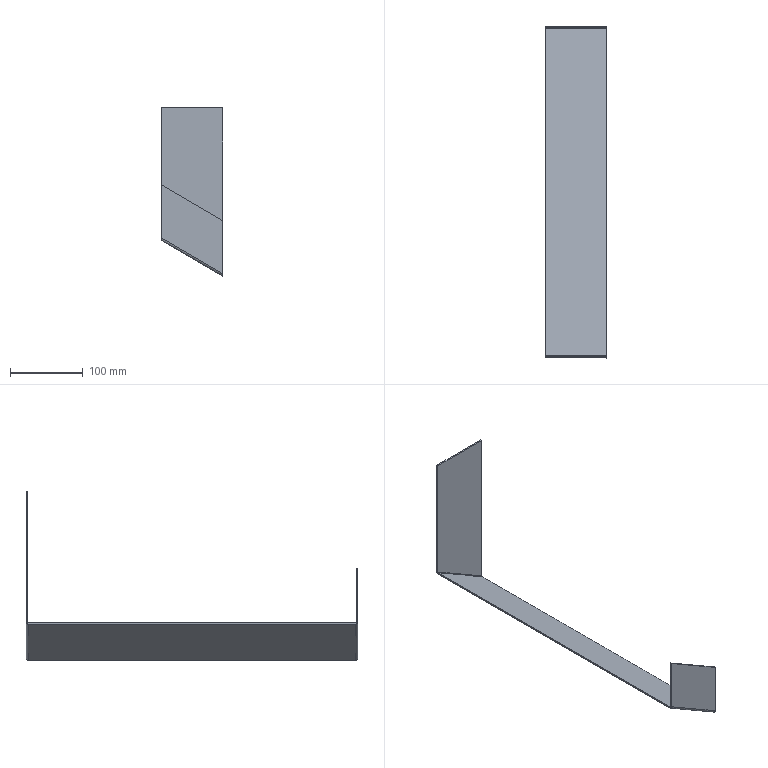Part | STEP file | lll_id4154_x_t | 1 solid | 14 faces | box 85 x 455 x 230.884 mm | volume 136229 mm3 | plane 10 | cylinder 4 | commonest cylinder face diameters 2 x2 6 x2
STEP:
#1=CARTESIAN_POINT('',(4052.435,-471.,-155.174));
#2=VERTEX_POINT('',#1);
#3=CARTESIAN_POINT('',(4052.435,-471.,-227.92));
#4=VERTEX_POINT('',#3);
#5=CARTESIAN_POINT('',(4052.435,-471.,-250.));
#6=DIRECTION('',(0.,0.,-1.));
#7=VECTOR('',#6,1.);
#8=LINE('',#5,#7);
#9=EDGE_CURVE('',#2,#4,#8,.T.);
#10=ORIENTED_EDGE('',*,*,#9,.T.);
#11=CARTESIAN_POINT('',(4052.435,-468.,-231.384));
#12=VERTEX_POINT('',#11);
#13=CARTESIAN_POINT('',(4052.435,-468.,-227.92));
#14=DIRECTION('',(1.,0.,0.));
#15=DIRECTION('',(0.,0.,-1.));
#16=AXIS2_PLACEMENT_3D('',#13,#14,#15);
#17=ELLIPSE('',#16,3.464,3.);
#18=EDGE_CURVE('',#4,#12,#17,.T.);
#19=ORIENTED_EDGE('',*,*,#18,.T.);
#20=CARTESIAN_POINT('',(4052.435,-19.,-231.384));
#21=VERTEX_POINT('',#20);
#22=CARTESIAN_POINT('',(4052.435,600.,-231.384));
#23=DIRECTION('',(0.,1.,0.));
#24=VECTOR('',#23,1.);
#25=LINE('',#22,#24);
#26=EDGE_CURVE('',#12,#21,#25,.T.);
#27=ORIENTED_EDGE('',*,*,#26,.T.);
#28=CARTESIAN_POINT('',(4052.435,-16.,-227.92));
#29=VERTEX_POINT('',#28);
#30=CARTESIAN_POINT('',(4052.435,-19.,-227.92));
#31=DIRECTION('',(1.,0.,0.));
#32=DIRECTION('',(0.,0.,-1.));
#33=AXIS2_PLACEMENT_3D('',#30,#31,#32);
#34=ELLIPSE('',#33,3.464,3.);
#35=EDGE_CURVE('',#21,#29,#34,.T.);
#36=ORIENTED_EDGE('',*,*,#35,.T.);
#37=CARTESIAN_POINT('',(4052.435,-16.,-0.5));
#38=VERTEX_POINT('',#37);
#39=CARTESIAN_POINT('',(4052.435,-16.,-131.405));
#40=DIRECTION('',(0.,0.,-1.));
#41=VECTOR('',#40,1.);
#42=LINE('',#39,#41);
#43=EDGE_CURVE('',#38,#29,#42,.T.);
#44=ORIENTED_EDGE('',*,*,#43,.F.);
#45=CARTESIAN_POINT('',(4052.435,-18.,-0.5));
#46=VERTEX_POINT('',#45);
#47=CARTESIAN_POINT('',(4052.435,-16.,-0.5));
#48=DIRECTION('',(0.,1.,0.));
#49=VECTOR('',#48,1.);
#50=LINE('',#47,#49);
#51=EDGE_CURVE('',#46,#38,#50,.T.);
#52=ORIENTED_EDGE('',*,*,#51,.F.);
#53=CARTESIAN_POINT('',(4052.435,-18.,-227.92));
#54=VERTEX_POINT('',#53);
#55=CARTESIAN_POINT('',(4052.435,-18.,-250.));
#56=DIRECTION('',(0.,0.,1.));
#57=VECTOR('',#56,1.);
#58=LINE('',#55,#57);
#59=EDGE_CURVE('',#54,#46,#58,.T.);
#60=ORIENTED_EDGE('',*,*,#59,.F.);
#61=CARTESIAN_POINT('',(4052.435,-19.,-229.075));
#62=VERTEX_POINT('',#61);
#63=CARTESIAN_POINT('',(4052.435,-19.,-227.92));
#64=DIRECTION('',(-1.,0.,0.));
#65=DIRECTION('',(0.,0.,1.));
#66=AXIS2_PLACEMENT_3D('',#63,#64,#65);
#67=ELLIPSE('',#66,1.155,1.);
#68=EDGE_CURVE('',#54,#62,#67,.T.);
#69=ORIENTED_EDGE('',*,*,#68,.T.);
#70=CARTESIAN_POINT('',(4052.435,-468.,-229.075));
#71=VERTEX_POINT('',#70);
#72=CARTESIAN_POINT('',(4052.435,600.,-229.075));
#73=DIRECTION('',(0.,1.,0.));
#74=VECTOR('',#73,1.);
#75=LINE('',#72,#74);
#76=EDGE_CURVE('',#71,#62,#75,.T.);
#77=ORIENTED_EDGE('',*,*,#76,.F.);
#78=CARTESIAN_POINT('',(4052.435,-469.,-227.92));
#79=VERTEX_POINT('',#78);
#80=CARTESIAN_POINT('',(4052.435,-468.,-227.92));
#81=DIRECTION('',(-1.,0.,0.));
#82=DIRECTION('',(0.,0.,1.));
#83=AXIS2_PLACEMENT_3D('',#80,#81,#82);
#84=ELLIPSE('',#83,1.155,1.);
#85=EDGE_CURVE('',#71,#79,#84,.T.);
#86=ORIENTED_EDGE('',*,*,#85,.T.);
#87=CARTESIAN_POINT('',(4052.435,-469.,-155.174));
#88=VERTEX_POINT('',#87);
#89=CARTESIAN_POINT('',(4052.435,-469.,-180.));
#90=DIRECTION('',(0.,0.,1.));
#91=VECTOR('',#90,1.);
#92=LINE('',#89,#91);
#93=EDGE_CURVE('',#79,#88,#92,.T.);
#94=ORIENTED_EDGE('',*,*,#93,.T.);
#95=CARTESIAN_POINT('',(4052.435,0.,-155.174));
#96=DIRECTION('',(0.,-1.,0.));
#97=VECTOR('',#96,1.);
#98=LINE('',#95,#97);
#99=EDGE_CURVE('',#88,#2,#98,.T.);
#100=ORIENTED_EDGE('',*,*,#99,.T.);
#101=EDGE_LOOP('',(#10,#19,#27,#36,#44,#52,#60,#69,#77,#86,#94,#100));
#102=FACE_OUTER_BOUND('',#101,.T.);
#103=CARTESIAN_POINT('',(4052.435,0.,-250.));
#104=DIRECTION('',(1.,0.,0.));
#105=DIRECTION('',(0.,0.,-1.));
#106=AXIS2_PLACEMENT_3D('',#103,#104,#105);
#107=PLANE('',#106);
#108=ADVANCED_FACE('',(#102),#107,.T.);
#109=CARTESIAN_POINT('',(3967.435,-19.,-182.309));
#110=VERTEX_POINT('',#109);
#111=CARTESIAN_POINT('',(3967.435,-468.,-182.309));
#112=VERTEX_POINT('',#111);
#113=CARTESIAN_POINT('',(3967.435,600.,-182.309));
#114=DIRECTION('',(0.,-1.,0.));
#115=VECTOR('',#114,1.);
#116=LINE('',#113,#115);
#117=EDGE_CURVE('',#110,#112,#116,.T.);
#118=ORIENTED_EDGE('',*,*,#117,.T.);
#119=CARTESIAN_POINT('',(3967.435,-471.,-178.845));
#120=VERTEX_POINT('',#119);
#121=CARTESIAN_POINT('',(3967.435,-468.,-178.845));
#122=DIRECTION('',(-1.,0.,0.));
#123=DIRECTION('',(0.,0.,-1.));
#124=AXIS2_PLACEMENT_3D('',#121,#122,#123);
#125=ELLIPSE('',#124,3.464,3.);
#126=EDGE_CURVE('',#112,#120,#125,.T.);
#127=ORIENTED_EDGE('',*,*,#126,.T.);
#128=CARTESIAN_POINT('',(3967.435,-471.,-106.099));
#129=VERTEX_POINT('',#128);
#130=CARTESIAN_POINT('',(3967.435,-471.,-180.));
#131=DIRECTION('',(0.,0.,-1.));
#132=VECTOR('',#131,1.);
#133=LINE('',#130,#132);
#134=EDGE_CURVE('',#129,#120,#133,.T.);
#135=ORIENTED_EDGE('',*,*,#134,.F.);
#136=CARTESIAN_POINT('',(3967.435,-469.,-106.099));
#137=VERTEX_POINT('',#136);
#138=CARTESIAN_POINT('',(3967.435,0.,-106.099));
#139=DIRECTION('',(0.,1.,0.));
#140=VECTOR('',#139,1.);
#141=LINE('',#138,#140);
#142=EDGE_CURVE('',#129,#137,#141,.T.);
#143=ORIENTED_EDGE('',*,*,#142,.T.);
#144=CARTESIAN_POINT('',(3967.435,-469.,-178.845));
#145=VERTEX_POINT('',#144);
#146=CARTESIAN_POINT('',(3967.435,-469.,-180.));
#147=DIRECTION('',(0.,0.,-1.));
#148=VECTOR('',#147,1.);
#149=LINE('',#146,#148);
#150=EDGE_CURVE('',#137,#145,#149,.T.);
#151=ORIENTED_EDGE('',*,*,#150,.T.);
#152=CARTESIAN_POINT('',(3967.435,-468.,-180.));
#153=VERTEX_POINT('',#152);
#154=CARTESIAN_POINT('',(3967.435,-468.,-178.845));
#155=DIRECTION('',(1.,0.,0.));
#156=DIRECTION('',(0.,0.,1.));
#157=AXIS2_PLACEMENT_3D('',#154,#155,#156);
#158=ELLIPSE('',#157,1.155,1.);
#159=EDGE_CURVE('',#145,#153,#158,.T.);
#160=ORIENTED_EDGE('',*,*,#159,.T.);
#161=CARTESIAN_POINT('',(3967.435,-19.,-180.));
#162=VERTEX_POINT('',#161);
#163=CARTESIAN_POINT('',(3967.435,600.,-180.));
#164=DIRECTION('',(0.,-1.,0.));
#165=VECTOR('',#164,1.);
#166=LINE('',#163,#165);
#167=EDGE_CURVE('',#162,#153,#166,.T.);
#168=ORIENTED_EDGE('',*,*,#167,.F.);
#169=CARTESIAN_POINT('',(3967.435,-18.,-178.845));
#170=VERTEX_POINT('',#169);
#171=CARTESIAN_POINT('',(3967.435,-19.,-178.845));
#172=DIRECTION('',(1.,0.,0.));
#173=DIRECTION('',(0.,0.,1.));
#174=AXIS2_PLACEMENT_3D('',#171,#172,#173);
#175=ELLIPSE('',#174,1.155,1.);
#176=EDGE_CURVE('',#162,#170,#175,.T.);
#177=ORIENTED_EDGE('',*,*,#176,.T.);
#178=CARTESIAN_POINT('',(3967.435,-18.,-0.5));
#179=VERTEX_POINT('',#178);
#180=CARTESIAN_POINT('',(3967.435,-18.,-0.5));
#181=DIRECTION('',(0.,0.,-1.));
#182=VECTOR('',#181,1.);
#183=LINE('',#180,#182);
#184=EDGE_CURVE('',#179,#170,#183,.T.);
#185=ORIENTED_EDGE('',*,*,#184,.F.);
#186=CARTESIAN_POINT('',(3967.435,-16.,-0.5));
#187=VERTEX_POINT('',#186);
#188=CARTESIAN_POINT('',(3967.435,-5.,-0.5));
#189=DIRECTION('',(0.,-1.,0.));
#190=VECTOR('',#189,1.);
#191=LINE('',#188,#190);
#192=EDGE_CURVE('',#187,#179,#191,.T.);
#193=ORIENTED_EDGE('',*,*,#192,.F.);
#194=CARTESIAN_POINT('',(3967.435,-16.,-178.845));
#195=VERTEX_POINT('',#194);
#196=CARTESIAN_POINT('',(3967.435,-16.,-0.5));
#197=DIRECTION('',(0.,0.,-1.));
#198=VECTOR('',#197,1.);
#199=LINE('',#196,#198);
#200=EDGE_CURVE('',#187,#195,#199,.T.);
#201=ORIENTED_EDGE('',*,*,#200,.T.);
#202=CARTESIAN_POINT('',(3967.435,-16.172,-180.));
#203=VERTEX_POINT('',#202);
#204=CARTESIAN_POINT('',(3967.435,-19.,-178.845));
#205=DIRECTION('',(-1.,0.,0.));
#206=DIRECTION('',(0.,0.,-1.));
#207=AXIS2_PLACEMENT_3D('',#204,#205,#206);
#208=ELLIPSE('',#207,3.464,3.);
#209=EDGE_CURVE('',#195,#203,#208,.T.);
#210=ORIENTED_EDGE('',*,*,#209,.T.);
#211=CARTESIAN_POINT('',(3967.435,-18.,-180.));
#212=VERTEX_POINT('',#211);
#213=CARTESIAN_POINT('',(3967.435,600.,-180.));
#214=DIRECTION('',(0.,-1.,0.));
#215=VECTOR('',#214,1.);
#216=LINE('',#213,#215);
#217=EDGE_CURVE('',#203,#212,#216,.T.);
#218=ORIENTED_EDGE('',*,*,#217,.T.);
#219=ORIENTED_EDGE('',*,*,#217,.F.);
#220=CARTESIAN_POINT('',(3967.435,-19.,-178.845));
#221=DIRECTION('',(-1.,0.,0.));
#222=DIRECTION('',(0.,0.,-1.));
#223=AXIS2_PLACEMENT_3D('',#220,#221,#222);
#224=ELLIPSE('',#223,3.464,3.);
#225=EDGE_CURVE('',#203,#110,#224,.T.);
#226=ORIENTED_EDGE('',*,*,#225,.T.);
#227=EDGE_LOOP('',(#118,#127,#135,#143,#151,#160,#168,#177,#185,#193,#201,#210,#218,#219,#226));
#228=FACE_OUTER_BOUND('',#227,.T.);
#229=CARTESIAN_POINT('',(3967.435,0.,-160.));
#230=DIRECTION('',(1.,0.,0.));
#231=DIRECTION('',(0.,0.,-1.));
#232=AXIS2_PLACEMENT_3D('',#229,#230,#231);
#233=PLANE('',#232);
#234=ADVANCED_FACE('',(#228),#233,.F.);
#235=ORIENTED_EDGE('',*,*,#26,.F.);
#236=CARTESIAN_POINT('',(3966.435,-468.,-181.732));
#237=DIRECTION('',(-0.866,0.,0.5));
#238=VECTOR('',#237,1.);
#239=LINE('',#236,#238);
#240=EDGE_CURVE('',#12,#112,#239,.T.);
#241=ORIENTED_EDGE('',*,*,#240,.T.);
#242=ORIENTED_EDGE('',*,*,#117,.F.);
#243=CARTESIAN_POINT('',(4052.435,-19.,-231.384));
#244=DIRECTION('',(0.866,0.,-0.5));
#245=VECTOR('',#244,1.);
#246=LINE('',#243,#245);
#247=EDGE_CURVE('',#110,#21,#246,.T.);
#248=ORIENTED_EDGE('',*,*,#247,.T.);
#249=EDGE_LOOP('',(#235,#241,#242,#248));
#250=FACE_OUTER_BOUND('',#249,.T.);
#251=CARTESIAN_POINT('',(3966.435,600.,-181.732));
#252=DIRECTION('',(0.5,0.,0.866));
#253=DIRECTION('',(0.866,0.,-0.5));
#254=AXIS2_PLACEMENT_3D('',#251,#252,#253);
#255=PLANE('',#254);
#256=ADVANCED_FACE('',(#250),#255,.F.);
#257=ORIENTED_EDGE('',*,*,#134,.T.);
#258=CARTESIAN_POINT('',(3967.935,-471.,-179.134));
#259=DIRECTION('',(0.866,0.,-0.5));
#260=VECTOR('',#259,1.);
#261=LINE('',#258,#260);
#262=EDGE_CURVE('',#120,#4,#261,.T.);
#263=ORIENTED_EDGE('',*,*,#262,.T.);
#264=ORIENTED_EDGE('',*,*,#9,.F.);
#265=CARTESIAN_POINT('',(3999.435,-471.,-124.574));
#266=DIRECTION('',(0.866,0.,-0.5));
#267=VECTOR('',#266,1.);
#268=LINE('',#265,#267);
#269=EDGE_CURVE('',#129,#2,#268,.T.);
#270=ORIENTED_EDGE('',*,*,#269,.F.);
#271=EDGE_LOOP('',(#257,#263,#264,#270));
#272=FACE_OUTER_BOUND('',#271,.T.);
#273=CARTESIAN_POINT('',(3967.435,-471.,-180.));
#274=DIRECTION('',(0.,1.,0.));
#275=DIRECTION('',(-0.866,0.,0.5));
#276=AXIS2_PLACEMENT_3D('',#273,#274,#275);
#277=PLANE('',#276);
#278=ADVANCED_FACE('',(#272),#277,.F.);
#279=ORIENTED_EDGE('',*,*,#269,.T.);
#280=ORIENTED_EDGE('',*,*,#99,.F.);
#281=CARTESIAN_POINT('',(3999.435,-469.,-124.574));
#282=DIRECTION('',(0.866,0.,-0.5));
#283=VECTOR('',#282,1.);
#284=LINE('',#281,#283);
#285=EDGE_CURVE('',#137,#88,#284,.T.);
#286=ORIENTED_EDGE('',*,*,#285,.F.);
#287=ORIENTED_EDGE('',*,*,#142,.F.);
#288=EDGE_LOOP('',(#279,#280,#286,#287));
#289=FACE_OUTER_BOUND('',#288,.T.);
#290=CARTESIAN_POINT('',(3999.435,-471.,-124.574));
#291=DIRECTION('',(-0.5,0.,-0.866));
#292=DIRECTION('',(-0.866,0.,0.5));
#293=AXIS2_PLACEMENT_3D('',#290,#291,#292);
#294=PLANE('',#293);
#295=ADVANCED_FACE('',(#289),#294,.F.);
#296=ORIENTED_EDGE('',*,*,#167,.T.);
#297=CARTESIAN_POINT('',(4052.435,-468.,-229.075));
#298=DIRECTION('',(0.866,0.,-0.5));
#299=VECTOR('',#298,1.);
#300=LINE('',#297,#299);
#301=EDGE_CURVE('',#153,#71,#300,.T.);
#302=ORIENTED_EDGE('',*,*,#301,.T.);
#303=ORIENTED_EDGE('',*,*,#76,.T.);
#304=CARTESIAN_POINT('',(3967.435,-19.,-180.));
#305=DIRECTION('',(-0.866,0.,0.5));
#306=VECTOR('',#305,1.);
#307=LINE('',#304,#306);
#308=EDGE_CURVE('',#62,#162,#307,.T.);
#309=ORIENTED_EDGE('',*,*,#308,.T.);
#310=EDGE_LOOP('',(#296,#302,#303,#309));
#311=FACE_OUTER_BOUND('',#310,.T.);
#312=CARTESIAN_POINT('',(3967.435,600.,-180.));
#313=DIRECTION('',(0.5,0.,0.866));
#314=DIRECTION('',(0.866,0.,-0.5));
#315=AXIS2_PLACEMENT_3D('',#312,#313,#314);
#316=PLANE('',#315);
#317=ADVANCED_FACE('',(#311),#316,.T.);
#318=ORIENTED_EDGE('',*,*,#184,.T.);
#319=CARTESIAN_POINT('',(3937.883,-18.,-161.783));
#320=DIRECTION('',(0.866,0.,-0.5));
#321=VECTOR('',#320,1.);
#322=LINE('',#319,#321);
#323=EDGE_CURVE('',#170,#54,#322,.T.);
#324=ORIENTED_EDGE('',*,*,#323,.T.);
#325=ORIENTED_EDGE('',*,*,#59,.T.);
#326=CARTESIAN_POINT('',(4031.,-18.,-0.5));
#327=DIRECTION('',(-1.,0.,0.));
#328=VECTOR('',#327,1.);
#329=LINE('',#326,#328);
#330=EDGE_CURVE('',#46,#179,#329,.T.);
#331=ORIENTED_EDGE('',*,*,#330,.T.);
#332=EDGE_LOOP('',(#318,#324,#325,#331));
#333=FACE_OUTER_BOUND('',#332,.T.);
#334=CARTESIAN_POINT('',(4031.,-18.,-0.5));
#335=DIRECTION('',(0.,1.,0.));
#336=DIRECTION('',(0.,0.,-1.));
#337=AXIS2_PLACEMENT_3D('',#334,#335,#336);
#338=PLANE('',#337);
#339=ADVANCED_FACE('',(#333),#338,.F.);
#340=ORIENTED_EDGE('',*,*,#330,.F.);
#341=ORIENTED_EDGE('',*,*,#51,.T.);
#342=CARTESIAN_POINT('',(4031.,-16.,-0.5));
#343=DIRECTION('',(-1.,0.,0.));
#344=VECTOR('',#343,1.);
#345=LINE('',#342,#344);
#346=EDGE_CURVE('',#38,#187,#345,.T.);
#347=ORIENTED_EDGE('',*,*,#346,.T.);
#348=ORIENTED_EDGE('',*,*,#192,.T.);
#349=EDGE_LOOP('',(#340,#341,#347,#348));
#350=FACE_OUTER_BOUND('',#349,.T.);
#351=CARTESIAN_POINT('',(4031.,-16.,-0.5));
#352=DIRECTION('',(0.,0.,1.));
#353=DIRECTION('',(-1.,0.,0.));
#354=AXIS2_PLACEMENT_3D('',#351,#352,#353);
#355=PLANE('',#354);
#356=ADVANCED_FACE('',(#350),#355,.T.);
#357=ORIENTED_EDGE('',*,*,#93,.F.);
#358=CARTESIAN_POINT('',(3967.935,-469.,-179.134));
#359=DIRECTION('',(-0.866,0.,0.5));
#360=VECTOR('',#359,1.);
#361=LINE('',#358,#360);
#362=EDGE_CURVE('',#79,#145,#361,.T.);
#363=ORIENTED_EDGE('',*,*,#362,.T.);
#364=ORIENTED_EDGE('',*,*,#150,.F.);
#365=ORIENTED_EDGE('',*,*,#285,.T.);
#366=EDGE_LOOP('',(#357,#363,#364,#365));
#367=FACE_OUTER_BOUND('',#366,.T.);
#368=CARTESIAN_POINT('',(3967.435,-469.,-180.));
#369=DIRECTION('',(0.,1.,0.));
#370=DIRECTION('',(-0.866,0.,0.5));
#371=AXIS2_PLACEMENT_3D('',#368,#369,#370);
#372=PLANE('',#371);
#373=ADVANCED_FACE('',(#367),#372,.T.);
#374=ORIENTED_EDGE('',*,*,#43,.T.);
#375=CARTESIAN_POINT('',(3968.935,-16.,-179.711));
#376=DIRECTION('',(-0.866,0.,0.5));
#377=VECTOR('',#376,1.);
#378=LINE('',#375,#377);
#379=EDGE_CURVE('',#29,#195,#378,.T.);
#380=ORIENTED_EDGE('',*,*,#379,.T.);
#381=ORIENTED_EDGE('',*,*,#200,.F.);
#382=ORIENTED_EDGE('',*,*,#346,.F.);
#383=EDGE_LOOP('',(#374,#380,#381,#382));
#384=FACE_OUTER_BOUND('',#383,.T.);
#385=CARTESIAN_POINT('',(4036.718,-16.,-131.405));
#386=DIRECTION('',(0.,1.,0.));
#387=DIRECTION('',(0.,0.,1.));
#388=AXIS2_PLACEMENT_3D('',#385,#386,#387);
#389=PLANE('',#388);
#390=ADVANCED_FACE('',(#384),#389,.T.);
#391=ORIENTED_EDGE('',*,*,#68,.F.);
#392=ORIENTED_EDGE('',*,*,#323,.F.);
#393=ORIENTED_EDGE('',*,*,#176,.F.);
#394=ORIENTED_EDGE('',*,*,#308,.F.);
#395=EDGE_LOOP('',(#391,#392,#393,#394));
#396=FACE_OUTER_BOUND('',#395,.T.);
#397=CARTESIAN_POINT('',(3967.935,-19.,-179.134));
#398=DIRECTION('',(-0.866,0.,0.5));
#399=DIRECTION('',(-0.5,0.,-0.866));
#400=AXIS2_PLACEMENT_3D('',#397,#398,#399);
#401=CYLINDRICAL_SURFACE('',#400,1.);
#402=ADVANCED_FACE('',(#396),#401,.F.);
#403=ORIENTED_EDGE('',*,*,#35,.F.);
#404=ORIENTED_EDGE('',*,*,#247,.F.);
#405=ORIENTED_EDGE('',*,*,#225,.F.);
#406=ORIENTED_EDGE('',*,*,#209,.F.);
#407=ORIENTED_EDGE('',*,*,#379,.F.);
#408=EDGE_LOOP('',(#403,#404,#405,#406,#407));
#409=FACE_OUTER_BOUND('',#408,.T.);
#410=CARTESIAN_POINT('',(3998.855,-19.,-196.985));
#411=DIRECTION('',(0.866,0.,-0.5));
#412=DIRECTION('',(0.5,0.,0.866));
#413=AXIS2_PLACEMENT_3D('',#410,#411,#412);
#414=CYLINDRICAL_SURFACE('',#413,3.);
#415=ADVANCED_FACE('',(#409),#414,.T.);
#416=ORIENTED_EDGE('',*,*,#159,.F.);
#417=ORIENTED_EDGE('',*,*,#362,.F.);
#418=ORIENTED_EDGE('',*,*,#85,.F.);
#419=ORIENTED_EDGE('',*,*,#301,.F.);
#420=EDGE_LOOP('',(#416,#417,#418,#419));
#421=FACE_OUTER_BOUND('',#420,.T.);
#422=CARTESIAN_POINT('',(3967.935,-468.,-179.134));
#423=DIRECTION('',(-0.866,0.,0.5));
#424=DIRECTION('',(-0.5,0.,-0.866));
#425=AXIS2_PLACEMENT_3D('',#422,#423,#424);
#426=CYLINDRICAL_SURFACE('',#425,1.);
#427=ADVANCED_FACE('',(#421),#426,.F.);
#428=ORIENTED_EDGE('',*,*,#126,.F.);
#429=ORIENTED_EDGE('',*,*,#240,.F.);
#430=ORIENTED_EDGE('',*,*,#18,.F.);
#431=ORIENTED_EDGE('',*,*,#262,.F.);
#432=EDGE_LOOP('',(#428,#429,#430,#431));
#433=FACE_OUTER_BOUND('',#432,.T.);
#434=CARTESIAN_POINT('',(3967.935,-468.,-179.134));
#435=DIRECTION('',(0.866,0.,-0.5));
#436=DIRECTION('',(0.5,0.,0.866));
#437=AXIS2_PLACEMENT_3D('',#434,#435,#436);
#438=CYLINDRICAL_SURFACE('',#437,3.);
#439=ADVANCED_FACE('',(#433),#438,.T.);
#440=CLOSED_SHELL('',(#108,#234,#256,#278,#295,#317,#339,#356,#373,#390,#402,#415,#427,#439));
#441=MANIFOLD_SOLID_BREP('',#440);
#442=(LENGTH_UNIT()NAMED_UNIT(*)SI_UNIT(.MILLI.,.METRE.));
#443=UNCERTAINTY_MEASURE_WITH_UNIT(LENGTH_MEASURE(0.00002),#442,'','');
#444=(NAMED_UNIT(*)PLANE_ANGLE_UNIT()SI_UNIT($,.RADIAN.));
#445=PLANE_ANGLE_MEASURE_WITH_UNIT(PLANE_ANGLE_MEASURE(0.01745),#444);
#446=DIMENSIONAL_EXPONENTS(0.,0.,0.,0.,0.,0.,0.);
#447=(CONVERSION_BASED_UNIT('DEGREE',#445)NAMED_UNIT(#446)PLANE_ANGLE_UNIT());
#448=(NAMED_UNIT(*)SI_UNIT($,.STERADIAN.)SOLID_ANGLE_UNIT());
#449=(GEOMETRIC_REPRESENTATION_CONTEXT(3)GLOBAL_UNCERTAINTY_ASSIGNED_CONTEXT((#443))GLOBAL_UNIT_ASSIGNED_CONTEXT((#442,#447,#448))REPRESENTATION_CONTEXT('',''));
#450=ADVANCED_BREP_SHAPE_REPRESENTATION('',(#441),#449);